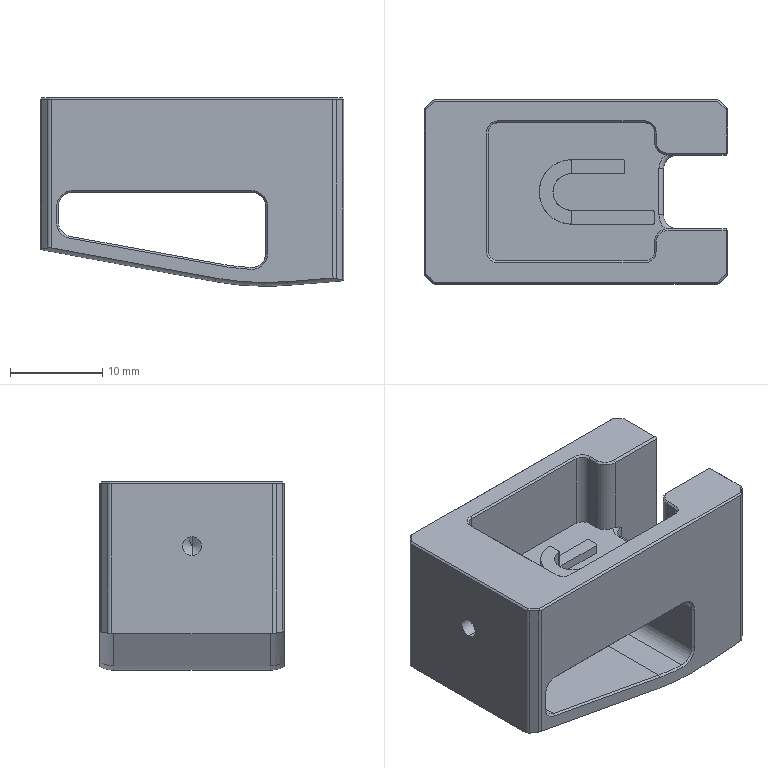NC program | NX | posted with a generic post | part box 33 x 20 x 20.478 mm
Lines 1 to 1200 of 3438:
N10 G17 G21 G94 G90
(PLANAR_MILL , TOOL : D4)
N12 T11 M6
N14 G54
N16 G17 G0 G90 X-12.4 Y-5.011 B0. C0. S9500 M3
N18 G43 Z30. H11
N20 Z1.5
N22 G94 G1 Y12.4 Z0.588 F1000.
N24 X-13.078 Z0.552
N26 X-16.011 Y-3.591 Z-0.3
N28 X-14.236 Y-3.893
N30 G3 X-14.271 Y-4.1 R24.1 F2200.
N32 G1 X-14.2
N34 Y-3.686
N36 G3 X-14.236 Y-3.893 R24.1
N38 G1 X-16.011 Y-3.591
N40 G3 X-16.298 Y-5.9 R25.9
N42 G1 X-12.4
N44 Y12.4
N46 X-13.078
N48 X-15.953 Y-3.263
N50 G3 X-16.011 Y-3.591 R25.9
N52 G1 Z1.2
N54 G0 X-12.4 Y-5.011
N56 G1 Y12.4 Z0.288 F1000.
N58 X-13.078 Z0.252
N60 X-16.011 Y-3.591 Z-0.6
N62 X-14.236 Y-3.893
N64 G3 X-14.271 Y-4.1 R24.1 F2200.
N66 G1 X-14.2
N68 Y-3.686
N70 G3 X-14.236 Y-3.893 R24.1
N72 G1 X-16.011 Y-3.591
N74 G3 X-16.298 Y-5.9 R25.9
N76 G1 X-12.4
N78 Y12.4
N80 X-13.078
N82 X-15.953 Y-3.263
N84 G3 X-16.011 Y-3.591 R25.9
N86 G1 Z0.9
N88 G0 X-12.4 Y-5.011
N90 G1 Y12.4 Z-0.012 F1000.
N92 X-13.078 Z-0.048
N94 X-16.011 Y-3.591 Z-0.9
N96 X-14.236 Y-3.893
N98 G3 X-14.271 Y-4.1 R24.1 F2200.
N100 G1 X-14.2
N102 Y-3.686
N104 G3 X-14.236 Y-3.893 R24.1
N106 G1 X-16.011 Y-3.591
N108 G3 X-16.298 Y-5.9 R25.9
N110 G1 X-12.4
N112 Y12.4
N114 X-13.078
N116 X-15.953 Y-3.263
N118 G3 X-16.011 Y-3.591 R25.9
N120 G1 Z0.6
N122 G0 X-12.4 Y-5.011
N124 G1 Y12.4 Z-0.312 F1000.
N126 X-13.078 Z-0.348
N128 X-16.011 Y-3.591 Z-1.2
N130 X-14.236 Y-3.893
N132 G3 X-14.271 Y-4.1 R24.1 F2200.
N134 G1 X-14.2
N136 Y-3.686
N138 G3 X-14.236 Y-3.893 R24.1
N140 G1 X-16.011 Y-3.591
N142 G3 X-16.298 Y-5.9 R25.9
N144 G1 X-12.4
N146 Y12.4
N148 X-13.078
N150 X-15.953 Y-3.263
N152 G3 X-16.011 Y-3.591 R25.9
N154 G1 Z0.3
N156 G0 X-12.4 Y-5.011
N158 G1 Y12.4 Z-0.612 F1000.
N160 X-13.078 Z-0.648
N162 X-16.011 Y-3.591 Z-1.5
N164 X-14.236 Y-3.893
N166 G3 X-14.271 Y-4.1 R24.1 F2200.
N168 G1 X-14.2
N170 Y-3.686
N172 G3 X-14.236 Y-3.893 R24.1
N174 G1 X-16.011 Y-3.591
N176 G3 X-16.298 Y-5.9 R25.9
N178 G1 X-12.4
N180 Y12.4
N182 X-13.078
N184 X-15.953 Y-3.263
N186 G3 X-16.011 Y-3.591 R25.9
N188 G1 Z0.
N190 G0 X-12.4 Y-5.011
N192 G1 Y12.4 Z-0.912 F1000.
N194 X-13.078 Z-0.948
N196 X-16.011 Y-3.591 Z-1.8
N198 X-14.236 Y-3.893
N200 G3 X-14.271 Y-4.1 R24.1 F2200.
N202 G1 X-14.2
N204 Y-3.686
N206 G3 X-14.236 Y-3.893 R24.1
N208 G1 X-16.011 Y-3.591
N210 G3 X-16.298 Y-5.9 R25.9
N212 G1 X-12.4
N214 Y12.4
N216 X-13.078
N218 X-15.953 Y-3.263
N220 G3 X-16.011 Y-3.591 R25.9
N222 G1 Z-0.3
N224 G0 X-12.4 Y-5.011
N226 G1 Y12.4 Z-1.212 F1000.
N228 X-13.078 Z-1.248
N230 X-16.011 Y-3.591 Z-2.1
N232 X-14.236 Y-3.893
N234 G3 X-14.271 Y-4.1 R24.1 F2200.
N236 G1 X-14.2
N238 Y-3.686
N240 G3 X-14.236 Y-3.893 R24.1
N242 G1 X-16.011 Y-3.591
N244 G3 X-16.298 Y-5.9 R25.9
N246 G1 X-12.4
N248 Y12.4
N250 X-13.078
N252 X-15.953 Y-3.263
N254 G3 X-16.011 Y-3.591 R25.9
N256 G1 Z-0.6
N258 G0 X-12.4 Y-5.011
N260 G1 Y12.4 Z-1.512 F1000.
N262 X-13.078 Z-1.548
N264 X-16.011 Y-3.591 Z-2.4
N266 X-14.236 Y-3.893
N268 G3 X-14.271 Y-4.1 R24.1 F2200.
N270 G1 X-14.2
N272 Y-3.686
N274 G3 X-14.236 Y-3.893 R24.1
N276 G1 X-16.011 Y-3.591
N278 G3 X-16.298 Y-5.9 R25.9
N280 G1 X-12.4
N282 Y12.4
N284 X-13.078
N286 X-15.953 Y-3.263
N288 G3 X-16.011 Y-3.591 R25.9
N290 G1 Z-0.9
N292 G0 X-12.4 Y-5.011
N294 G1 Y12.4 Z-1.812 F1000.
N296 X-13.078 Z-1.848
N298 X-16.011 Y-3.591 Z-2.7
N300 X-14.236 Y-3.893
N302 G3 X-14.271 Y-4.1 R24.1 F2200.
N304 G1 X-14.2
N306 Y-3.686
N308 G3 X-14.236 Y-3.893 R24.1
N310 G1 X-16.011 Y-3.591
N312 G3 X-16.298 Y-5.9 R25.9
N314 G1 X-12.4
N316 Y12.4
N318 X-13.078
N320 X-15.953 Y-3.263
N322 G3 X-16.011 Y-3.591 R25.9
N324 G1 Z-1.2
N326 G0 X-12.4 Y-5.011
N328 G1 Y12.4 Z-2.112 F1000.
N330 X-13.078 Z-2.148
N332 X-16.011 Y-3.591 Z-3.
N334 X-14.236 Y-3.893
N336 G3 X-14.271 Y-4.1 R24.1 F2200.
N338 G1 X-14.2
N340 Y-3.686
N342 G3 X-14.236 Y-3.893 R24.1
N344 G1 X-16.011 Y-3.591
N346 G3 X-16.298 Y-5.9 R25.9
N348 G1 X-12.4
N350 Y12.4
N352 X-13.078
N354 X-15.953 Y-3.263
N356 G3 X-16.011 Y-3.591 R25.9
N358 G1 Z-1.5
N360 G0 X-12.4 Y-5.011
N362 G1 Y12.4 Z-2.412 F1000.
N364 X-13.078 Z-2.448
N366 X-16.011 Y-3.591 Z-3.3
N368 X-14.236 Y-3.893
N370 G3 X-14.271 Y-4.1 R24.1 F2200.
N372 G1 X-14.2
N374 Y-3.686
N376 G3 X-14.236 Y-3.893 R24.1
N378 G1 X-16.011 Y-3.591
N380 G3 X-16.298 Y-5.9 R25.9
N382 G1 X-12.4
N384 Y12.4
N386 X-13.078
N388 X-15.953 Y-3.263
N390 G3 X-16.011 Y-3.591 R25.9
N392 G1 Z-1.8
N394 G0 X-12.4 Y-5.011
N396 G1 Y12.4 Z-2.712 F1000.
N398 X-13.078 Z-2.748
N400 X-16.011 Y-3.591 Z-3.6
N402 X-14.236 Y-3.893
N404 G3 X-14.271 Y-4.1 R24.1 F2200.
N406 G1 X-14.2
N408 Y-3.686
N410 G3 X-14.236 Y-3.893 R24.1
N412 G1 X-16.011 Y-3.591
N414 G3 X-16.298 Y-5.9 R25.9
N416 G1 X-12.4
N418 Y12.4
N420 X-13.078
N422 X-15.953 Y-3.263
N424 G3 X-16.011 Y-3.591 R25.9
N426 G1 Z-2.1
N428 G0 X-12.4 Y-5.011
N430 G1 Y12.4 Z-3.012 F1000.
N432 X-13.078 Z-3.048
N434 X-16.011 Y-3.591 Z-3.9
N436 X-14.236 Y-3.893
N438 G3 X-14.271 Y-4.1 R24.1 F2200.
N440 G1 X-14.2
N442 Y-3.686
N444 G3 X-14.236 Y-3.893 R24.1
N446 G1 X-16.011 Y-3.591
N448 G3 X-16.298 Y-5.9 R25.9
N450 G1 X-12.4
N452 Y12.4
N454 X-13.078
N456 X-15.953 Y-3.263
N458 G3 X-16.011 Y-3.591 R25.9
N460 G1 Z-2.4
N462 G0 X-12.4 Y-5.011
N464 G1 Y12.4 Z-3.312 F1000.
N466 X-13.078 Z-3.348
N468 X-16.011 Y-3.591 Z-4.2
N470 X-14.236 Y-3.893
N472 G3 X-14.271 Y-4.1 R24.1 F2200.
N474 G1 X-14.2
N476 Y-3.686
N478 G3 X-14.236 Y-3.893 R24.1
N480 G1 X-16.011 Y-3.591
N482 G3 X-16.298 Y-5.9 R25.9
N484 G1 X-12.4
N486 Y12.4
N488 X-13.078
N490 X-15.953 Y-3.263
N492 G3 X-16.011 Y-3.591 R25.9
N494 G1 Z-2.7
N496 G0 X-12.4 Y-5.011
N498 G1 Y12.4 Z-3.612 F1000.
N500 X-13.078 Z-3.648
N502 X-16.011 Y-3.591 Z-4.5
N504 X-14.236 Y-3.893
N506 G3 X-14.271 Y-4.1 R24.1 F2200.
N508 G1 X-14.2
N510 Y-3.686
N512 G3 X-14.236 Y-3.893 R24.1
N514 G1 X-16.011 Y-3.591
N516 G3 X-16.298 Y-5.9 R25.9
N518 G1 X-12.4
N520 Y12.4
N522 X-13.078
N524 X-15.953 Y-3.263
N526 G3 X-16.011 Y-3.591 R25.9
N528 G1 Z-3.
N530 G0 X-12.4 Y-5.011
N532 G1 Y12.4 Z-3.912 F1000.
N534 X-13.078 Z-3.948
N536 X-16.011 Y-3.591 Z-4.8
N538 X-14.236 Y-3.893
N540 G3 X-14.271 Y-4.1 R24.1 F2200.
N542 G1 X-14.2
N544 Y-3.686
N546 G3 X-14.236 Y-3.893 R24.1
N548 G1 X-16.011 Y-3.591
N550 G3 X-16.298 Y-5.9 R25.9
N552 G1 X-12.4
N554 Y12.4
N556 X-13.078
N558 X-15.953 Y-3.263
N560 G3 X-16.011 Y-3.591 R25.9
N562 G1 Z-3.3
N564 G0 X-12.4 Y-5.011
N566 G1 Y12.4 Z-4.212 F1000.
N568 X-13.078 Z-4.248
N570 X-16.011 Y-3.591 Z-5.1
N572 X-14.236 Y-3.893
N574 G3 X-14.271 Y-4.1 R24.1 F2200.
N576 G1 X-14.2
N578 Y-3.686
N580 G3 X-14.236 Y-3.893 R24.1
N582 G1 X-16.011 Y-3.591
N584 G3 X-16.298 Y-5.9 R25.9
N586 G1 X-12.4
N588 Y12.4
N590 X-13.078
N592 X-15.953 Y-3.263
N594 G3 X-16.011 Y-3.591 R25.9
N596 G1 Z-3.6
N598 G0 X-12.4 Y-5.011
N600 G1 Y12.4 Z-4.512 F1000.
N602 X-13.078 Z-4.548
N604 X-16.011 Y-3.591 Z-5.4
N606 X-14.236 Y-3.893
N608 G3 X-14.271 Y-4.1 R24.1 F2200.
N610 G1 X-14.2
N612 Y-3.686
N614 G3 X-14.236 Y-3.893 R24.1
N616 G1 X-16.011 Y-3.591
N618 G3 X-16.298 Y-5.9 R25.9
N620 G1 X-12.4
N622 Y12.4
N624 X-13.078
N626 X-15.953 Y-3.263
N628 G3 X-16.011 Y-3.591 R25.9
N630 G1 Z-3.9
N632 G0 X-12.4 Y-5.011
N634 G1 Y12.4 Z-4.812 F1000.
N636 X-13.078 Z-4.848
N638 X-16.011 Y-3.591 Z-5.7
N640 X-14.236 Y-3.893
N642 G3 X-14.271 Y-4.1 R24.1 F2200.
N644 G1 X-14.2
N646 Y-3.686
N648 G3 X-14.236 Y-3.893 R24.1
N650 G1 X-16.011 Y-3.591
N652 G3 X-16.298 Y-5.9 R25.9
N654 G1 X-12.4
N656 Y12.4
N658 X-13.078
N660 X-15.953 Y-3.263
N662 G3 X-16.011 Y-3.591 R25.9
N664 G1 Z-4.2
N666 G0 X-12.4 Y-5.011
N668 G1 Y12.4 Z-5.112 F1000.
N670 X-13.078 Z-5.148
N672 X-16.011 Y-3.591 Z-6.
N674 X-14.236 Y-3.893
N676 G3 X-14.271 Y-4.1 R24.1 F2200.
N678 G1 X-14.2
N680 Y-3.686
N682 G3 X-14.236 Y-3.893 R24.1
N684 G1 X-16.011 Y-3.591
N686 G3 X-16.298 Y-5.9 R25.9
N688 G1 X-12.4
N690 Y12.4
N692 X-13.078
N694 X-15.953 Y-3.263
N696 G3 X-16.011 Y-3.591 R25.9
N698 G1 Z-4.5
N700 G0 X-12.4 Y-5.011
N702 G1 Y12.4 Z-5.412 F1000.
N704 X-13.078 Z-5.448
N706 X-16.011 Y-3.591 Z-6.3
N708 X-14.236 Y-3.893
N710 G3 X-14.271 Y-4.1 R24.1 F2200.
N712 G1 X-14.2
N714 Y-3.686
N716 G3 X-14.236 Y-3.893 R24.1
N718 G1 X-16.011 Y-3.591
N720 G3 X-16.298 Y-5.9 R25.9
N722 G1 X-12.4
N724 Y12.4
N726 X-13.078
N728 X-15.953 Y-3.263
N730 G3 X-16.011 Y-3.591 R25.9
N732 G1 Z-4.8
N734 G0 X-12.4 Y-5.011
N736 G1 Y12.4 Z-5.712 F1000.
N738 X-13.078 Z-5.748
N740 X-16.011 Y-3.591 Z-6.6
N742 X-14.236 Y-3.893
N744 G3 X-14.271 Y-4.1 R24.1 F2200.
N746 G1 X-14.2
N748 Y-3.686
N750 G3 X-14.236 Y-3.893 R24.1
N752 G1 X-16.011 Y-3.591
N754 G3 X-16.298 Y-5.9 R25.9
N756 G1 X-12.4
N758 Y12.4
N760 X-13.078
N762 X-15.953 Y-3.263
N764 G3 X-16.011 Y-3.591 R25.9
N766 G1 Z-5.1
N768 G0 X-12.4 Y-5.011
N770 G1 Y12.4 Z-6.012 F1000.
N772 X-13.078 Z-6.048
N774 X-16.011 Y-3.591 Z-6.9
N776 X-14.236 Y-3.893
N778 G3 X-14.271 Y-4.1 R24.1 F2200.
N780 G1 X-14.2
N782 Y-3.686
N784 G3 X-14.236 Y-3.893 R24.1
N786 G1 X-16.011 Y-3.591
N788 G3 X-16.298 Y-5.9 R25.9
N790 G1 X-12.4
N792 Y12.4
N794 X-13.078
N796 X-15.953 Y-3.263
N798 G3 X-16.011 Y-3.591 R25.9
N800 G1 Z-5.4
N802 G0 X-12.4 Y-5.011
N804 G1 Y12.4 Z-6.312 F1000.
N806 X-13.078 Z-6.348
N808 X-16.011 Y-3.591 Z-7.2
N810 X-14.236 Y-3.893
N812 G3 X-14.271 Y-4.1 R24.1 F2200.
N814 G1 X-14.2
N816 Y-3.686
N818 G3 X-14.236 Y-3.893 R24.1
N820 G1 X-16.011 Y-3.591
N822 G3 X-16.298 Y-5.9 R25.9
N824 G1 X-12.4
N826 Y12.4
N828 X-13.078
N830 X-15.953 Y-3.263
N832 G3 X-16.011 Y-3.591 R25.9
N834 G1 Z-5.7
N836 G0 X-12.4 Y-5.011
N838 G1 Y12.4 Z-6.612 F1000.
N840 X-13.078 Z-6.648
N842 X-16.011 Y-3.591 Z-7.5
N844 X-14.236 Y-3.893
N846 G3 X-14.271 Y-4.1 R24.1 F2200.
N848 G1 X-14.2
N850 Y-3.686
N852 G3 X-14.236 Y-3.893 R24.1
N854 G1 X-16.011 Y-3.591
N856 G3 X-16.298 Y-5.9 R25.9
N858 G1 X-12.4
N860 Y12.4
N862 X-13.078
N864 X-15.953 Y-3.263
N866 G3 X-16.011 Y-3.591 R25.9
N868 G1 Z-6.
N870 G0 X-12.4 Y-5.011
N872 G1 Y12.4 Z-6.912 F1000.
N874 X-13.078 Z-6.948
N876 X-16.011 Y-3.591 Z-7.8
N878 X-14.236 Y-3.893
N880 G3 X-14.271 Y-4.1 R24.1 F2200.
N882 G1 X-14.2
N884 Y-3.686
N886 G3 X-14.236 Y-3.893 R24.1
N888 G1 X-16.011 Y-3.591
N890 G3 X-16.298 Y-5.9 R25.9
N892 G1 X-12.4
N894 Y12.4
N896 X-13.078
N898 X-15.953 Y-3.263
N900 G3 X-16.011 Y-3.591 R25.9
N902 G1 Z-6.3
N904 G0 X-12.4 Y-5.011
N906 G1 Y12.4 Z-7.212 F1000.
N908 X-13.078 Z-7.248
N910 X-16.011 Y-3.591 Z-8.1
N912 X-14.236 Y-3.893
N914 G3 X-14.271 Y-4.1 R24.1 F2200.
N916 G1 X-14.2
N918 Y-3.686
N920 G3 X-14.236 Y-3.893 R24.1
N922 G1 X-16.011 Y-3.591
N924 G3 X-16.298 Y-5.9 R25.9
N926 G1 X-12.4
N928 Y12.4
N930 X-13.078
N932 X-15.953 Y-3.263
N934 G3 X-16.011 Y-3.591 R25.9
N936 G1 Z-6.6
N938 G0 X-12.4 Y-5.011
N940 G1 Y12.4 Z-7.512 F1000.
N942 X-13.078 Z-7.548
N944 X-16.011 Y-3.591 Z-8.4
N946 X-14.236 Y-3.893
N948 G3 X-14.271 Y-4.1 R24.1 F2200.
N950 G1 X-14.2
N952 Y-3.686
N954 G3 X-14.236 Y-3.893 R24.1
N956 G1 X-16.011 Y-3.591
N958 G3 X-16.298 Y-5.9 R25.9
N960 G1 X-12.4
N962 Y12.4
N964 X-13.078
N966 X-15.953 Y-3.263
N968 G3 X-16.011 Y-3.591 R25.9
N970 G1 Z-6.9
N972 G0 X-12.4 Y-5.011
N974 G1 Y12.4 Z-7.812 F1000.
N976 X-13.078 Z-7.848
N978 X-16.011 Y-3.591 Z-8.7
N980 X-14.236 Y-3.893
N982 G3 X-14.271 Y-4.1 R24.1 F2200.
N984 G1 X-14.2
N986 Y-3.686
N988 G3 X-14.236 Y-3.893 R24.1
N990 G1 X-16.011 Y-3.591
N992 G3 X-16.298 Y-5.9 R25.9
N994 G1 X-12.4
N996 Y12.4
N998 X-13.078
N1000 X-15.953 Y-3.263
N1002 G3 X-16.011 Y-3.591 R25.9
N1004 G1 Z-7.2
N1006 G0 X-12.4 Y-5.011
N1008 G1 Y12.4 Z-8.112 F1000.
N1010 X-13.078 Z-8.148
N1012 X-16.011 Y-3.591 Z-9.
N1014 X-14.236 Y-3.893
N1016 G3 X-14.271 Y-4.1 R24.1 F2200.
N1018 G1 X-14.2
N1020 Y-3.686
N1022 G3 X-14.236 Y-3.893 R24.1
N1024 G1 X-16.011 Y-3.591
N1026 G3 X-16.298 Y-5.9 R25.9
N1028 G1 X-12.4
N1030 Y12.4
N1032 X-13.078
N1034 X-15.953 Y-3.263
N1036 G3 X-16.011 Y-3.591 R25.9
N1038 G1 Z-7.5
N1040 G0 X-12.4 Y-5.011
N1042 G1 Y12.4 Z-8.412 F1000.
N1044 X-13.078 Z-8.448
N1046 X-16.011 Y-3.591 Z-9.3
N1048 X-14.236 Y-3.893
N1050 G3 X-14.271 Y-4.1 R24.1 F2200.
N1052 G1 X-14.2
N1054 Y-3.686
N1056 G3 X-14.236 Y-3.893 R24.1
N1058 G1 X-16.011 Y-3.591
N1060 G3 X-16.298 Y-5.9 R25.9
N1062 G1 X-12.4
N1064 Y12.4
N1066 X-13.078
N1068 X-15.953 Y-3.263
N1070 G3 X-16.011 Y-3.591 R25.9
N1072 G1 Z-7.8
N1074 G0 X-12.4 Y-5.011
N1076 G1 Y12.4 Z-8.712 F1000.
N1078 X-13.078 Z-8.748
N1080 X-16.011 Y-3.591 Z-9.6
N1082 X-14.236 Y-3.893
N1084 G3 X-14.271 Y-4.1 R24.1 F2200.
N1086 G1 X-14.2
N1088 Y-3.686
N1090 G3 X-14.236 Y-3.893 R24.1
N1092 G1 X-16.011 Y-3.591
N1094 G3 X-16.298 Y-5.9 R25.9
N1096 G1 X-12.4
N1098 Y12.4
N1100 X-13.078
N1102 X-15.953 Y-3.263
N1104 G3 X-16.011 Y-3.591 R25.9
N1106 G1 Z-8.1
N1108 G0 X-12.4 Y-5.011
N1110 G1 Y12.4 Z-9.012 F1000.
N1112 X-13.078 Z-9.048
N1114 X-16.011 Y-3.591 Z-9.9
N1116 X-14.236 Y-3.893
N1118 G3 X-14.271 Y-4.1 R24.1 F2200.
N1120 G1 X-14.2
N1122 Y-3.686
N1124 G3 X-14.236 Y-3.893 R24.1
N1126 G1 X-16.011 Y-3.591
N1128 G3 X-16.298 Y-5.9 R25.9
N1130 G1 X-12.4
N1132 Y12.4
N1134 X-13.078
N1136 X-15.953 Y-3.263
N1138 G3 X-16.011 Y-3.591 R25.9
N1140 G1 Z-8.4
N1142 G0 X-12.4 Y-5.011
N1144 G1 Y12.4 Z-9.312 F1000.
N1146 X-13.078 Z-9.348
N1148 X-16.011 Y-3.591 Z-10.2
N1150 X-14.236 Y-3.893
N1152 G3 X-14.271 Y-4.1 R24.1 F2200.
N1154 G1 X-14.2
N1156 Y-3.686
N1158 G3 X-14.236 Y-3.893 R24.1
N1160 G1 X-16.011 Y-3.591
N1162 G3 X-16.298 Y-5.9 R25.9
N1164 G1 X-12.4
N1166 Y12.4
N1168 X-13.078
N1170 X-15.953 Y-3.263
N1172 G3 X-16.011 Y-3.591 R25.9
N1174 G1 Z-8.7
N1176 G0 X-12.4 Y-5.011
N1178 G1 Y12.4 Z-9.612 F1000.
N1180 X-13.078 Z-9.648
N1182 X-16.011 Y-3.591 Z-10.5
N1184 X-14.236 Y-3.893
N1186 G3 X-14.271 Y-4.1 R24.1 F2200.
N1188 G1 X-14.2
N1190 Y-3.686
N1192 G3 X-14.236 Y-3.893 R24.1
N1194 G1 X-16.011 Y-3.591
N1196 G3 X-16.298 Y-5.9 R25.9
N1198 G1 X-12.4
N1200 Y12.4
N1202 X-13.078
N1204 X-15.953 Y-3.263
N1206 G3 X-16.011 Y-3.591 R25.9
N1208 G1 Z-9.
N1210 G0 X-12.4 Y-5.011
N1212 G1 Y12.4 Z-9.912 F1000.
N1214 X-13.078 Z-9.948
N1216 X-16.011 Y-3.591 Z-10.8
N1218 X-14.236 Y-3.893
N1220 G3 X-14.271 Y-4.1 R24.1 F2200.
N1222 G1 X-14.2
N1224 Y-3.686
N1226 G3 X-14.236 Y-3.893 R24.1
N1228 G1 X-16.011 Y-3.591
N1230 G3 X-16.298 Y-5.9 R25.9
N1232 G1 X-12.4
N1234 Y12.4
N1236 X-13.078
N1238 X-15.953 Y-3.263
N1240 G3 X-16.011 Y-3.591 R25.9
N1242 G1 Z-9.3
N1244 G0 X-12.4 Y-5.011
N1246 G1 Y12.4 Z-10.212 F1000.
N1248 X-13.078 Z-10.248
N1250 X-16.011 Y-3.591 Z-11.1
N1252 X-14.236 Y-3.893
N1254 G3 X-14.271 Y-4.1 R24.1 F2200.
N1256 G1 X-14.2
N1258 Y-3.686
N1260 G3 X-14.236 Y-3.893 R24.1
N1262 G1 X-16.011 Y-3.591
N1264 G3 X-16.298 Y-5.9 R25.9
N1266 G1 X-12.4
N1268 Y12.4
N1270 X-13.078
N1272 X-15.953 Y-3.263
N1274 G3 X-16.011 Y-3.591 R25.9
N1276 G1 Z-9.6
N1278 G0 X-12.4 Y-5.011
N1280 G1 Y12.4 Z-10.512 F1000.
N1282 X-13.078 Z-10.548
N1284 X-16.011 Y-3.591 Z-11.4
N1286 X-14.236 Y-3.893
N1288 G3 X-14.271 Y-4.1 R24.1 F2200.
N1290 G1 X-14.2
N1292 Y-3.686
N1294 G3 X-14.236 Y-3.893 R24.1
N1296 G1 X-16.011 Y-3.591
N1298 G3 X-16.298 Y-5.9 R25.9
N1300 G1 X-12.4
N1302 Y12.4
N1304 X-13.078
N1306 X-15.953 Y-3.263
N1308 G3 X-16.011 Y-3.591 R25.9
N1310 G1 Z-9.9
N1312 G0 X-12.4 Y-5.011
N1314 G1 Y12.4 Z-10.812 F1000.
N1316 X-13.078 Z-10.848
N1318 X-16.011 Y-3.591 Z-11.7
N1320 X-14.236 Y-3.893
N1322 G3 X-14.271 Y-4.1 R24.1 F2200.
N1324 G1 X-14.2
N1326 Y-3.686
N1328 G3 X-14.236 Y-3.893 R24.1
N1330 G1 X-16.011 Y-3.591
N1332 G3 X-16.298 Y-5.9 R25.9
N1334 G1 X-12.4
N1336 Y12.4
N1338 X-13.078
N1340 X-15.953 Y-3.263
N1342 G3 X-16.011 Y-3.591 R25.9
N1344 G1 Z-10.2
N1346 G0 X-12.4 Y-5.011
N1348 G1 Y12.4 Z-11.112 F1000.
N1350 X-13.078 Z-11.148
N1352 X-16.011 Y-3.591 Z-12.
N1354 X-14.236 Y-3.893
N1356 G3 X-14.271 Y-4.1 R24.1 F2200.
N1358 G1 X-14.2
N1360 Y-3.686
N1362 G3 X-14.236 Y-3.893 R24.1
N1364 G1 X-16.011 Y-3.591
N1366 G3 X-16.298 Y-5.9 R25.9
N1368 G1 X-12.4
N1370 Y12.4
N1372 X-13.078
N1374 X-15.953 Y-3.263
N1376 G3 X-16.011 Y-3.591 R25.9
N1378 G1 Z-10.5
N1380 G0 X-12.4 Y-5.011
N1382 G1 Y12.4 Z-11.412 F1000.
N1384 X-13.078 Z-11.448
N1386 X-16.011 Y-3.591 Z-12.3
N1388 X-14.236 Y-3.893
N1390 G3 X-14.271 Y-4.1 R24.1 F2200.
N1392 G1 X-14.2
N1394 Y-3.686
N1396 G3 X-14.236 Y-3.893 R24.1
N1398 G1 X-16.011 Y-3.591
N1400 G3 X-16.298 Y-5.9 R25.9
N1402 G1 X-12.4
N1404 Y12.4
N1406 X-13.078
N1408 X-15.953 Y-3.263
N1410 G3 X-16.011 Y-3.591 R25.9
N1412 G1 Z-10.8
N1414 G0 X-12.4 Y-5.011
N1416 G1 Y12.4 Z-11.712 F1000.
N1418 X-13.078 Z-11.748
N1420 X-16.011 Y-3.591 Z-12.6
N1422 X-14.236 Y-3.893
N1424 G3 X-14.271 Y-4.1 R24.1 F2200.
N1426 G1 X-14.2
N1428 Y-3.686
N1430 G3 X-14.236 Y-3.893 R24.1
N1432 G1 X-16.011 Y-3.591
N1434 G3 X-16.298 Y-5.9 R25.9
N1436 G1 X-12.4
N1438 Y12.4
N1440 X-13.078
N1442 X-15.953 Y-3.263
N1444 G3 X-16.011 Y-3.591 R25.9
N1446 G1 Z-11.1
N1448 G0 X-12.4 Y-5.011
N1450 G1 Y12.4 Z-12.012 F1000.
N1452 X-13.078 Z-12.048
N1454 X-16.011 Y-3.591 Z-12.9
N1456 X-14.236 Y-3.893
N1458 G3 X-14.271 Y-4.1 R24.1 F2200.
N1460 G1 X-14.2
N1462 Y-3.686
N1464 G3 X-14.236 Y-3.893 R24.1
N1466 G1 X-16.011 Y-3.591
N1468 G3 X-16.298 Y-5.9 R25.9
N1470 G1 X-12.4
N1472 Y12.4
N1474 X-13.078
N1476 X-15.953 Y-3.263
N1478 G3 X-16.011 Y-3.591 R25.9
N1480 G1 Z-11.4
N1482 G0 X-12.4 Y-5.011
N1484 G1 Y12.4 Z-12.312 F1000.
N1486 X-13.078 Z-12.348
N1488 X-16.011 Y-3.591 Z-13.2
N1490 X-14.236 Y-3.893
N1492 G3 X-14.271 Y-4.1 R24.1 F2200.
N1494 G1 X-14.2
N1496 Y-3.686
N1498 G3 X-14.236 Y-3.893 R24.1
N1500 G1 X-16.011 Y-3.591
N1502 G3 X-16.298 Y-5.9 R25.9
N1504 G1 X-12.4
N1506 Y12.4
N1508 X-13.078
N1510 X-15.953 Y-3.263
N1512 G3 X-16.011 Y-3.591 R25.9
N1514 G1 Z-11.7
N1516 G0 X-12.4 Y-5.011
N1518 G1 Y12.4 Z-12.612 F1000.
N1520 X-13.078 Z-12.648
N1522 X-16.011 Y-3.591 Z-13.5
N1524 X-14.236 Y-3.893
N1526 G3 X-14.271 Y-4.1 R24.1 F2200.
N1528 G1 X-14.2
N1530 Y-3.686
N1532 G3 X-14.236 Y-3.893 R24.1
N1534 G1 X-16.011 Y-3.591
N1536 G3 X-16.298 Y-5.9 R25.9
N1538 G1 X-12.4
N1540 Y12.4
N1542 X-13.078
N1544 X-15.953 Y-3.263
N1546 G3 X-16.011 Y-3.591 R25.9
N1548 G1 Z-12.
N1550 G0 X-12.4 Y-5.011
N1552 G1 Y12.4 Z-12.912 F1000.
N1554 X-13.078 Z-12.948
N1556 X-16.011 Y-3.591 Z-13.8
N1558 X-14.236 Y-3.893
N1560 G3 X-14.271 Y-4.1 R24.1 F2200.
N1562 G1 X-14.2
N1564 Y-3.686
N1566 G3 X-14.236 Y-3.893 R24.1
N1568 G1 X-16.011 Y-3.591
N1570 G3 X-16.298 Y-5.9 R25.9
N1572 G1 X-12.4
N1574 Y12.4
N1576 X-13.078
N1578 X-15.953 Y-3.263
N1580 G3 X-16.011 Y-3.591 R25.9
N1582 G1 Z-12.3
N1584 G0 X-12.4 Y-5.011
N1586 G1 Y12.4 Z-13.212 F1000.
N1588 X-13.078 Z-13.248
N1590 X-16.011 Y-3.591 Z-14.1
N1592 X-14.236 Y-3.893
N1594 G3 X-14.271 Y-4.1 R24.1 F2200.
N1596 G1 X-14.2
N1598 Y-3.686
N1600 G3 X-14.236 Y-3.893 R24.1
N1602 G1 X-16.011 Y-3.591
N1604 G3 X-16.298 Y-5.9 R25.9
N1606 G1 X-12.4
N1608 Y12.4
N1610 X-13.078
N1612 X-15.953 Y-3.263
N1614 G3 X-16.011 Y-3.591 R25.9
N1616 G1 Z-12.6
N1618 G0 X-12.4 Y-5.011
N1620 G1 Y12.4 Z-13.512 F1000.
N1622 X-13.078 Z-13.548
N1624 X-16.011 Y-3.591 Z-14.4
N1626 X-14.236 Y-3.893
N1628 G3 X-14.271 Y-4.1 R24.1 F2200.
N1630 G1 X-14.2
N1632 Y-3.686
N1634 G3 X-14.236 Y-3.893 R24.1
N1636 G1 X-16.011 Y-3.591
N1638 G3 X-16.298 Y-5.9 R25.9
N1640 G1 X-12.4
N1642 Y12.4
N1644 X-13.078
N1646 X-15.953 Y-3.263
N1648 G3 X-16.011 Y-3.591 R25.9
N1650 G1 Z-12.9
N1652 G0 X-12.4 Y-5.011
N1654 G1 Y12.4 Z-13.812 F1000.
N1656 X-13.078 Z-13.848
N1658 X-16.011 Y-3.591 Z-14.7
N1660 X-14.236 Y-3.893
N1662 G3 X-14.271 Y-4.1 R24.1 F2200.
N1664 G1 X-14.2
N1666 Y-3.686
N1668 G3 X-14.236 Y-3.893 R24.1
N1670 G1 X-16.011 Y-3.591
N1672 G3 X-16.298 Y-5.9 R25.9
N1674 G1 X-12.4
N1676 Y12.4
N1678 X-13.078
N1680 X-15.953 Y-3.263
N1682 G3 X-16.011 Y-3.591 R25.9
N1684 G1 Z-13.2
N1686 G0 X-12.4 Y-5.011
N1688 G1 Y12.4 Z-14.112 F1000.
N1690 X-13.078 Z-14.148
N1692 X-16.011 Y-3.591 Z-15.
N1694 X-14.236 Y-3.893
N1696 G3 X-14.271 Y-4.1 R24.1 F2200.
N1698 G1 X-14.2
N1700 Y-3.686
N1702 G3 X-14.236 Y-3.893 R24.1
N1704 G1 X-16.011 Y-3.591
N1706 G3 X-16.298 Y-5.9 R25.9
N1708 G1 X-12.4
N1710 Y12.4
N1712 X-13.078
N1714 X-15.953 Y-3.263
N1716 G3 X-16.011 Y-3.591 R25.9
N1718 G1 Z-13.5
N1720 G0 X-12.4 Y-5.011
N1722 G1 Y12.4 Z-14.412 F1000.
N1724 X-13.078 Z-14.448
N1726 X-16.011 Y-3.591 Z-15.3
N1728 X-14.236 Y-3.893
N1730 G3 X-14.271 Y-4.1 R24.1 F2200.
N1732 G1 X-14.2
N1734 Y-3.686
N1736 G3 X-14.236 Y-3.893 R24.1
N1738 G1 X-16.011 Y-3.591
N1740 G3 X-16.298 Y-5.9 R25.9
N1742 G1 X-12.4
N1744 Y12.4
N1746 X-13.078
N1748 X-15.953 Y-3.263
N1750 G3 X-16.011 Y-3.591 R25.9
N1752 G1 Z-13.8
N1754 G0 X-12.4 Y-5.011
N1756 G1 Y12.4 Z-14.712 F1000.
N1758 X-13.078 Z-14.748
N1760 X-16.011 Y-3.591 Z-15.6
N1762 X-14.236 Y-3.893
N1764 G3 X-14.271 Y-4.1 R24.1 F2200.
N1766 G1 X-14.2
N1768 Y-3.686
N1770 G3 X-14.236 Y-3.893 R24.1
N1772 G1 X-16.011 Y-3.591
N1774 G3 X-16.298 Y-5.9 R25.9
N1776 G1 X-12.4
N1778 Y12.4
N1780 X-13.078
N1782 X-15.953 Y-3.263
N1784 G3 X-16.011 Y-3.591 R25.9
N1786 G1 Z-14.1
N1788 G0 X-12.4 Y-5.011
N1790 G1 Y12.4 Z-15.012 F1000.
N1792 X-13.078 Z-15.048
N1794 X-16.011 Y-3.591 Z-15.9
N1796 X-14.236 Y-3.893
N1798 G3 X-14.271 Y-4.1 R24.1 F2200.
N1800 G1 X-14.2
N1802 Y-3.686
N1804 G3 X-14.236 Y-3.893 R24.1
N1806 G1 X-16.011 Y-3.591
N1808 G3 X-16.298 Y-5.9 R25.9
N1810 G1 X-12.4
N1812 Y12.4
N1814 X-13.078
N1816 X-15.953 Y-3.263
N1818 G3 X-16.011 Y-3.591 R25.9
N1820 G1 Z-14.4
N1822 G0 X-12.4 Y-5.011
N1824 G1 Y12.4 Z-15.312 F1000.
N1826 X-13.078 Z-15.348
N1828 X-16.011 Y-3.591 Z-16.2
N1830 X-14.236 Y-3.893
N1832 G3 X-14.271 Y-4.1 R24.1 F2200.
N1834 G1 X-14.2
N1836 Y-3.686
N1838 G3 X-14.236 Y-3.893 R24.1
N1840 G1 X-16.011 Y-3.591
N1842 G3 X-16.298 Y-5.9 R25.9
N1844 G1 X-12.4
N1846 Y12.4
N1848 X-13.078
N1850 X-15.953 Y-3.263
N1852 G3 X-16.011 Y-3.591 R25.9
N1854 G1 Z-14.7
N1856 G0 X-12.4 Y-5.011
N1858 G1 Y12.4 Z-15.612 F1000.
N1860 X-13.078 Z-15.648
N1862 X-16.011 Y-3.591 Z-16.5
N1864 X-14.236 Y-3.893
N1866 G3 X-14.271 Y-4.1 R24.1 F2200.
N1868 G1 X-14.2
N1870 Y-3.686
N1872 G3 X-14.236 Y-3.893 R24.1
N1874 G1 X-16.011 Y-3.591
N1876 G3 X-16.298 Y-5.9 R25.9
N1878 G1 X-12.4
N1880 Y12.4
N1882 X-13.078
N1884 X-15.953 Y-3.263
N1886 G3 X-16.011 Y-3.591 R25.9
N1888 G1 Z-15.
N1890 G0 X-12.4 Y-5.011
N1892 G1 Y12.4 Z-15.912 F1000.
N1894 X-13.078 Z-15.948
N1896 X-16.011 Y-3.591 Z-16.8
N1898 X-14.236 Y-3.893
N1900 G3 X-14.271 Y-4.1 R24.1 F2200.
N1902 G1 X-14.2
N1904 Y-3.686
N1906 G3 X-14.236 Y-3.893 R24.1
N1908 G1 X-16.011 Y-3.591
N1910 G3 X-16.298 Y-5.9 R25.9
N1912 G1 X-12.4
N1914 Y12.4
N1916 X-13.078
N1918 X-15.953 Y-3.263
N1920 G3 X-16.011 Y-3.591 R25.9
N1922 G1 Z-15.3
N1924 G0 X-12.4 Y-5.011
N1926 G1 Y12.4 Z-16.212 F1000.
N1928 X-13.078 Z-16.248
N1930 X-16.011 Y-3.591 Z-17.1
N1932 X-14.236 Y-3.893
N1934 G3 X-14.271 Y-4.1 R24.1 F2200.
N1936 G1 X-14.2
N1938 Y-3.686
N1940 G3 X-14.236 Y-3.893 R24.1
N1942 G1 X-16.011 Y-3.591
N1944 G3 X-16.298 Y-5.9 R25.9
N1946 G1 X-12.4
N1948 Y12.4
N1950 X-13.078
N1952 X-15.953 Y-3.263
N1954 G3 X-16.011 Y-3.591 R25.9
N1956 G1 Z-15.6
N1958 G0 X-12.4 Y-5.011
N1960 G1 Y12.4 Z-16.512 F1000.
N1962 X-13.078 Z-16.548
N1964 X-16.011 Y-3.591 Z-17.4
N1966 X-14.236 Y-3.893
N1968 G3 X-14.271 Y-4.1 R24.1 F2200.
N1970 G1 X-14.2
N1972 Y-3.686
N1974 G3 X-14.236 Y-3.893 R24.1
N1976 G1 X-16.011 Y-3.591
N1978 G3 X-16.298 Y-5.9 R25.9
N1980 G1 X-12.4
N1982 Y12.4
N1984 X-13.078
N1986 X-15.953 Y-3.263
N1988 G3 X-16.011 Y-3.591 R25.9
N1990 G1 Z-15.9
N1992 G0 X-12.4 Y-5.011
N1994 G1 Y12.4 Z-16.812 F1000.
N1996 X-13.078 Z-16.848
N1998 X-16.011 Y-3.591 Z-17.7
N2000 X-14.236 Y-3.893
N2002 G3 X-14.271 Y-4.1 R24.1 F2200.
N2004 G1 X-14.2
N2006 Y-3.686
N2008 G3 X-14.236 Y-3.893 R24.1
N2010 G1 X-16.011 Y-3.591
N2012 G3 X-16.298 Y-5.9 R25.9
N2014 G1 X-12.4
N2016 Y12.4
N2018 X-13.078
N2020 X-15.953 Y-3.263
N2022 G3 X-16.011 Y-3.591 R25.9
N2024 G1 Z-16.2
N2026 G0 X-12.4 Y-5.011
N2028 G1 Y12.4 Z-17.112 F1000.
N2030 X-13.078 Z-17.148
N2032 X-16.011 Y-3.591 Z-18.
N2034 X-14.236 Y-3.893
N2036 G3 X-14.271 Y-4.1 R24.1 F2200.
N2038 G1 X-14.2
N2040 Y-3.686
N2042 G3 X-14.236 Y-3.893 R24.1
N2044 G1 X-16.011 Y-3.591
N2046 G3 X-16.298 Y-5.9 R25.9
N2048 G1 X-12.4
N2050 Y12.4
N2052 X-13.078
N2054 X-15.953 Y-3.263
N2056 G3 X-16.011 Y-3.591 R25.9
N2058 G1 Z-16.5
N2060 G0 X-12.4 Y-5.011
N2062 G1 Y12.4 Z-17.412 F1000.
N2064 X-13.078 Z-17.448
N2066 X-16.011 Y-3.591 Z-18.3
N2068 X-14.236 Y-3.893
N2070 G3 X-14.271 Y-4.1 R24.1 F2200.
N2072 G1 X-14.2
N2074 Y-3.686
N2076 G3 X-14.236 Y-3.893 R24.1
N2078 G1 X-16.011 Y-3.591
N2080 G3 X-16.298 Y-5.9 R25.9
N2082 G1 X-12.4
N2084 Y12.4
N2086 X-13.078
N2088 X-15.953 Y-3.263
N2090 G3 X-16.011 Y-3.591 R25.9
N2092 G1 Z-16.8
N2094 G0 X-12.4 Y-5.011
N2096 G1 Y12.4 Z-17.712 F1000.
N2098 X-13.078 Z-17.748
N2100 X-16.011 Y-3.591 Z-18.6
N2102 X-14.236 Y-3.893
N2104 G3 X-14.271 Y-4.1 R24.1 F2200.
N2106 G1 X-14.2
N2108 Y-3.686
N2110 G3 X-14.236 Y-3.893 R24.1
N2112 G1 X-16.011 Y-3.591
N2114 G3 X-16.298 Y-5.9 R25.9
N2116 G1 X-12.4
N2118 Y12.4
N2120 X-13.078
N2122 X-15.953 Y-3.263
N2124 G3 X-16.011 Y-3.591 R25.9
N2126 G1 Z-17.1
N2128 G0 X-12.4 Y-5.011
N2130 G1 Y12.4 Z-18.012 F1000.
N2132 X-13.078 Z-18.048
N2134 X-16.011 Y-3.591 Z-18.9
N2136 X-14.236 Y-3.893
N2138 G3 X-14.271 Y-4.1 R24.1 F2200.
N2140 G1 X-14.2
N2142 Y-3.686
N2144 G3 X-14.236 Y-3.893 R24.1
N2146 G1 X-16.011 Y-3.591
N2148 G3 X-16.298 Y-5.9 R25.9
N2150 G1 X-12.4
N2152 Y12.4
N2154 X-13.078
N2156 X-15.953 Y-3.263
N2158 G3 X-16.011 Y-3.591 R25.9
N2160 G1 Z-17.4
N2162 G0 X-12.4 Y-5.011
N2164 G1 Y12.4 Z-18.312 F1000.
N2166 X-13.078 Z-18.348
N2168 X-16.011 Y-3.591 Z-19.2
N2170 X-14.236 Y-3.893
N2172 G3 X-14.271 Y-4.1 R24.1 F2200.
N2174 G1 X-14.2
N2176 Y-3.686
N2178 G3 X-14.236 Y-3.893 R24.1
N2180 G1 X-16.011 Y-3.591
N2182 G3 X-16.298 Y-5.9 R25.9
N2184 G1 X-12.4
N2186 Y12.4
N2188 X-13.078
N2190 X-15.953 Y-3.263
N2192 G3 X-16.011 Y-3.591 R25.9
N2194 G1 Z-17.7
N2196 G0 X-12.4 Y-5.011
N2198 G1 Y12.4 Z-18.612 F1000.
N2200 X-13.078 Z-18.648
N2202 X-16.011 Y-3.591 Z-19.5
N2204 X-14.236 Y-3.893
N2206 G3 X-14.271 Y-4.1 R24.1 F2200.
N2208 G1 X-14.2
N2210 Y-3.686
N2212 G3 X-14.236 Y-3.893 R24.1
N2214 G1 X-16.011 Y-3.591
N2216 G3 X-16.298 Y-5.9 R25.9
N2218 G1 X-12.4
N2220 Y12.4
N2222 X-13.078
N2224 X-15.953 Y-3.263
N2226 G3 X-16.011 Y-3.591 R25.9
N2228 G1 Z-18.
N2230 G0 X-12.4 Y-5.011
N2232 G1 Y12.4 Z-18.912 F1000.
N2234 X-13.078 Z-18.948
N2236 X-16.011 Y-3.591 Z-19.8
N2238 X-14.236 Y-3.893
N2240 G3 X-14.271 Y-4.1 R24.1 F2200.
N2242 G1 X-14.2
N2244 Y-3.686
N2246 G3 X-14.236 Y-3.893 R24.1
N2248 G1 X-16.011 Y-3.591
N2250 G3 X-16.298 Y-5.9 R25.9
N2252 G1 X-12.4
N2254 Y12.4
N2256 X-13.078
N2258 X-15.953 Y-3.263
N2260 G3 X-16.011 Y-3.591 R25.9
N2262 G1 Z-18.3
N2264 G0 X-12.4 Y-3.103
N2266 G1 Y12.4 Z-19.112 F1000.
N2268 X-13.078 Z-19.148
N2270 X-16.011 Y-3.591 Z-20.
N2272 X-14.236 Y-3.893
N2274 G3 X-14.271 Y-4.1 R24.1 F2200.
N2276 G1 X-14.2
N2278 Y-3.686
N2280 G3 X-14.236 Y-3.893 R24.1
N2282 G1 X-16.011 Y-3.591
N2284 G3 X-16.298 Y-5.9 R25.9
N2286 G1 X-12.4
N2288 Y12.4
N2290 X-13.078
N2292 X-15.953 Y-3.263
N2294 G3 X-16.011 Y-3.591 R25.9
N2296 G1 Z-18.5
N2298 G0 Z30.
(PLANAR_MILL_COPY , TOOL : D4)
N2300 X-12.728 Y12.1
N2302 Z-4.
N2304 G1 Z-5. F1000.
N2306 Y12.25
N2308 G3 X-13.161 Y12.5 R0.5
N2310 G1 X-16.051 Y-3.245 F1200.
N2312 G3 X-16.406 Y-6. R26.
N2314 G1 X-12.3
N2316 Y12.5
N2318 X-13.161
N2320 G3 X-12.912 Y11.641 R1.
N2322 G1 Z-4.
N2324 G0 X-12.728 Y12.1 Z-9.
N2326 G1 Z-10. F1000.
N2328 Y12.25
N2330 G3 X-13.161 Y12.5 R0.5
N2332 G1 X-16.051 Y-3.245 F1200.
N2334 G3 X-16.406 Y-6. R26.
N2336 G1 X-12.3
N2338 Y12.5
N2340 X-13.161
N2342 G3 X-12.912 Y11.641 R1.
N2344 G1 Z-9.
N2346 G0 X-12.728 Y12.1 Z-14.
N2348 G1 Z-15. F1000.
N2350 Y12.25
N2352 G3 X-13.161 Y12.5 R0.5
N2354 G1 X-16.051 Y-3.245 F1200.
N2356 G3 X-16.406 Y-6. R26.
N2358 G1 X-12.3
N2360 Y12.5
N2362 X-13.161
N2364 G3 X-12.912 Y11.641 R1.
N2366 G1 Z-14.
N2368 G0 X-12.728 Y12.1 Z-19.
N2370 G1 Z-20. F1000.
N2372 Y12.25
N2374 G3 X-13.161 Y12.5 R0.5
N2376 G1 X-16.051 Y-3.245 F1200.
N2378 G3 X-16.406 Y-6. R26.
N2380 G1 X-12.3
N2382 Y12.5
N2384 X-13.161
N2386 G3 X-12.912 Y11.641 R1.
N2388 G1 Z-19.
N2390 G0 Z30.
N2392 M5